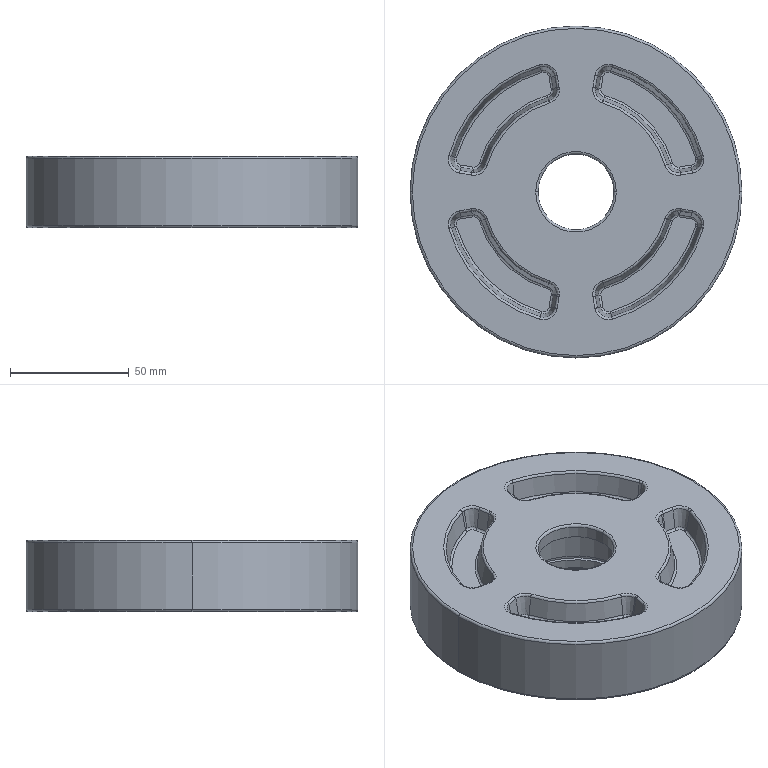Part | SolidWorks | features ICE 7, Fillet 2, CirPattern 1, Extrusion 1, MirrorPattern 1 | 1 solid | 267 faces | box 140 x 140 x 30 mm | volume 347987 mm3 | torus 120 | cone 64 | cylinder 50 | plane 33 | commonest cylinder face diameters 2 x32 3 x6 52 x4 32 x2 45 x2 55 x2